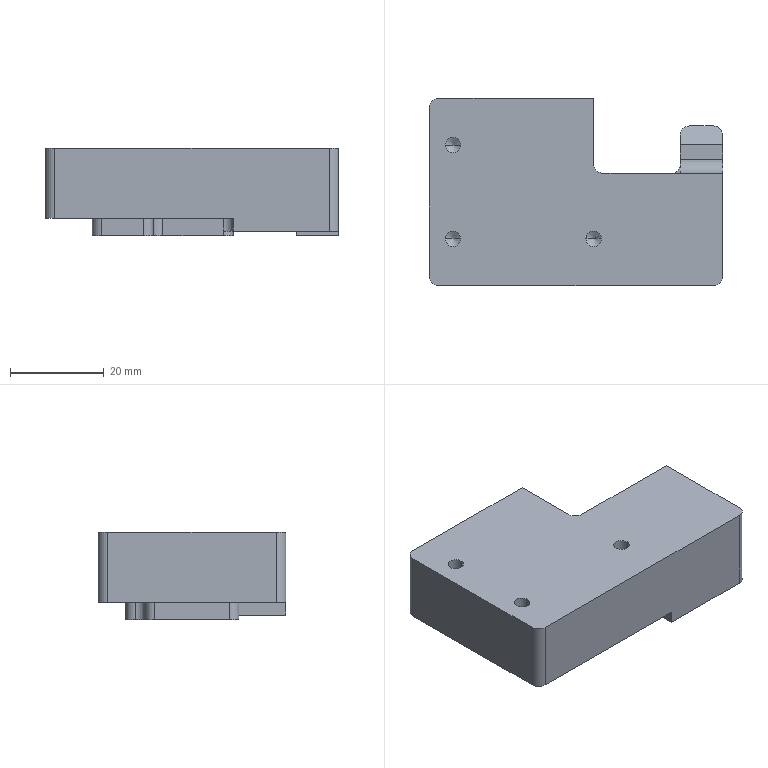Part | STEP file | 04-14-a pre-press block | 1 solid | 56 faces | box 62.5 x 40 x 18.7 mm | volume 34599 mm3 | plane 27 | cylinder 23 | cone 6 | commonest cylinder face diameters 4 x16 3.3 x6 6 x1